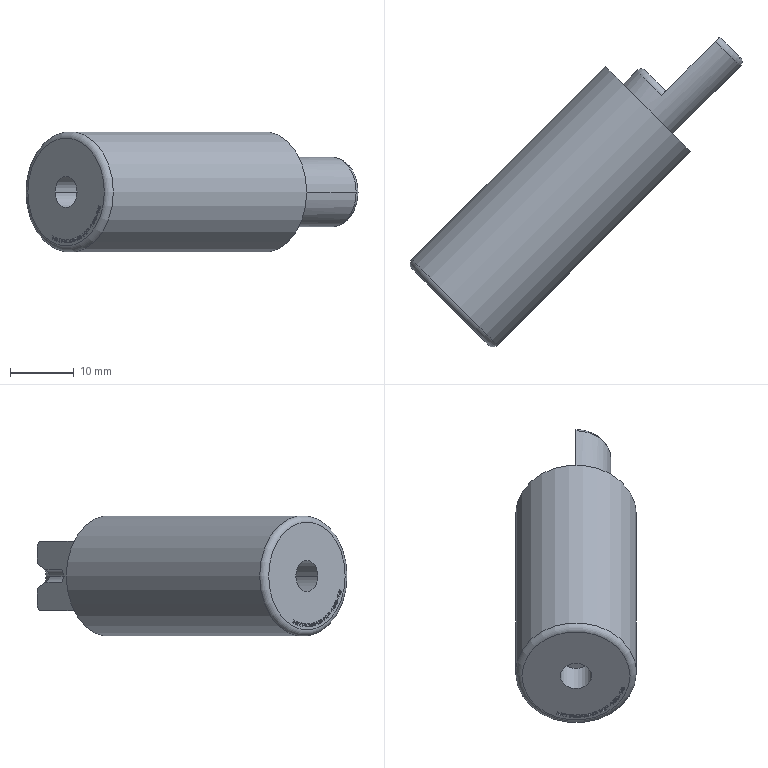Part | STEP file | 1_id1750_x_t | 1 solid | 157 faces | box 52.205 x 48.73 x 19 mm | volume 13276 mm3 | plane 112 | other 25 | cylinder 9 | cone 8 | torus 3 | commonest cylinder face diameters 2 x4 4.9 x2 11 x2 19 x1